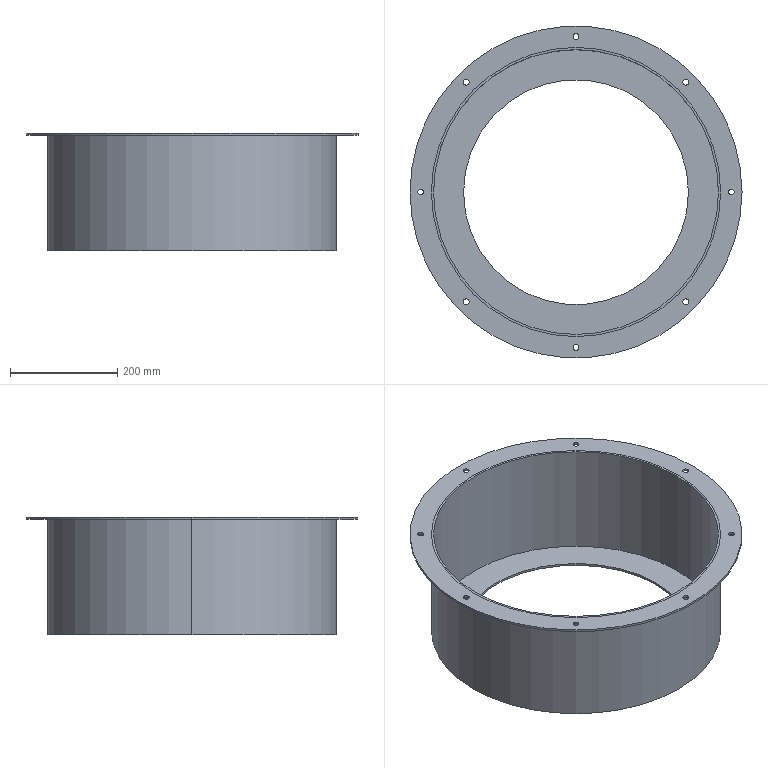Part | STEP file | Guard cover | 3 solids | 34 faces | box 620 x 620 x 220 mm | volume 2105294 mm3 | cylinder 28 | plane 6 | commonest cylinder face diameters 11 x16 532 x4 540 x4 420 x2 620 x2